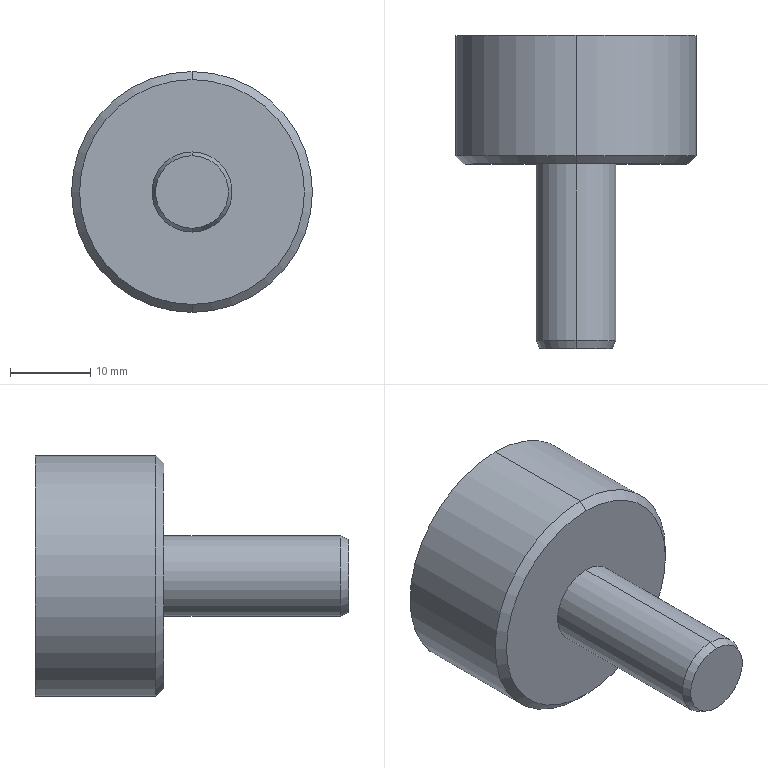Part | SolidWorks | features BaseBody 1 | 1 solid | 11 faces | box 30 x 39 x 30 mm | volume 13063 mm3 | cylinder 4 | cone 4 | plane 3 | commonest cylinder face diameters 10 x2 30 x2
STEP:
#1=CARTESIAN_POINT('',(418.,-39.,232.121));
#2=VERTEX_POINT('',#1);
#3=CARTESIAN_POINT('',(418.,-39.,262.121));
#4=VERTEX_POINT('',#3);
#5=CARTESIAN_POINT('',(418.,-39.,247.121));
#6=DIRECTION('',(0.,-1.,0.));
#7=DIRECTION('',(0.,0.,-1.));
#8=AXIS2_PLACEMENT_3D('',#5,#6,#7);
#9=CIRCLE('',#8,15.);
#10=EDGE_CURVE('',#2,#4,#9,.T.);
#11=ORIENTED_EDGE('',*,*,#10,.T.);
#12=CARTESIAN_POINT('',(418.,-54.,262.121));
#13=VERTEX_POINT('',#12);
#14=CARTESIAN_POINT('',(418.,-78.,262.121));
#15=DIRECTION('',(0.,-1.,0.));
#16=VECTOR('',#15,1000.);
#17=LINE('',#14,#16);
#18=EDGE_CURVE('',#4,#13,#17,.T.);
#19=ORIENTED_EDGE('',*,*,#18,.T.);
#20=CARTESIAN_POINT('',(418.,-54.,232.121));
#21=VERTEX_POINT('',#20);
#22=CARTESIAN_POINT('',(418.,-54.,247.121));
#23=DIRECTION('',(0.,1.,0.));
#24=DIRECTION('',(0.,0.,-1.));
#25=AXIS2_PLACEMENT_3D('',#22,#23,#24);
#26=CIRCLE('',#25,15.);
#27=EDGE_CURVE('',#13,#21,#26,.T.);
#28=ORIENTED_EDGE('',*,*,#27,.T.);
#29=CARTESIAN_POINT('',(418.,-78.,232.121));
#30=DIRECTION('',(0.,-1.,0.));
#31=VECTOR('',#30,1000.);
#32=LINE('',#29,#31);
#33=EDGE_CURVE('',#2,#21,#32,.T.);
#34=ORIENTED_EDGE('',*,*,#33,.F.);
#35=EDGE_LOOP('',(#11,#19,#28,#34));
#36=FACE_OUTER_BOUND('',#35,.T.);
#37=CARTESIAN_POINT('',(418.,-78.,247.121));
#38=DIRECTION('',(0.,-1.,0.));
#39=DIRECTION('',(0.,0.,-1.));
#40=AXIS2_PLACEMENT_3D('',#37,#38,#39);
#41=CYLINDRICAL_SURFACE('',#40,15.);
#42=ADVANCED_FACE('',(#36),#41,.T.);
#43=CARTESIAN_POINT('',(418.,-55.,261.121));
#44=VERTEX_POINT('',#43);
#45=CARTESIAN_POINT('',(418.,-55.,233.121));
#46=VERTEX_POINT('',#45);
#47=CARTESIAN_POINT('',(418.,-55.,247.121));
#48=DIRECTION('',(0.,1.,0.));
#49=DIRECTION('',(0.,0.,1.));
#50=AXIS2_PLACEMENT_3D('',#47,#48,#49);
#51=CIRCLE('',#50,14.);
#52=EDGE_CURVE('',#44,#46,#51,.T.);
#53=ORIENTED_EDGE('',*,*,#52,.T.);
#54=CARTESIAN_POINT('',(418.,-54.,232.121));
#55=DIRECTION('',(0.,0.7071,-0.7071));
#56=VECTOR('',#55,1000.);
#57=LINE('',#54,#56);
#58=EDGE_CURVE('',#46,#21,#57,.T.);
#59=ORIENTED_EDGE('',*,*,#58,.T.);
#60=ORIENTED_EDGE('',*,*,#27,.F.);
#61=CARTESIAN_POINT('',(418.,-54.,262.121));
#62=DIRECTION('',(0.,0.7071,0.7071));
#63=VECTOR('',#62,1000.);
#64=LINE('',#61,#63);
#65=EDGE_CURVE('',#44,#13,#64,.T.);
#66=ORIENTED_EDGE('',*,*,#65,.F.);
#67=EDGE_LOOP('',(#53,#59,#60,#66));
#68=FACE_OUTER_BOUND('',#67,.T.);
#69=CARTESIAN_POINT('',(418.,-54.,247.121));
#70=DIRECTION('',(0.,1.,0.));
#71=DIRECTION('',(0.,0.,1.));
#72=AXIS2_PLACEMENT_3D('',#69,#70,#71);
#73=CONICAL_SURFACE('',#72,15.,0.7854);
#74=ADVANCED_FACE('',(#68),#73,.T.);
#75=CARTESIAN_POINT('',(418.,-55.,252.121));
#76=VERTEX_POINT('',#75);
#77=CARTESIAN_POINT('',(418.,-55.,242.121));
#78=VERTEX_POINT('',#77);
#79=CARTESIAN_POINT('',(418.,-55.,247.121));
#80=DIRECTION('',(0.,1.,0.));
#81=DIRECTION('',(0.,0.,-1.));
#82=AXIS2_PLACEMENT_3D('',#79,#80,#81);
#83=CIRCLE('',#82,5.);
#84=EDGE_CURVE('',#76,#78,#83,.T.);
#85=ORIENTED_EDGE('',*,*,#84,.F.);
#86=CARTESIAN_POINT('',(418.,-77.,252.121));
#87=VERTEX_POINT('',#86);
#88=CARTESIAN_POINT('',(418.,-78.,252.121));
#89=DIRECTION('',(0.,-1.,0.));
#90=VECTOR('',#89,1000.);
#91=LINE('',#88,#90);
#92=EDGE_CURVE('',#76,#87,#91,.T.);
#93=ORIENTED_EDGE('',*,*,#92,.T.);
#94=CARTESIAN_POINT('',(418.,-77.,242.121));
#95=VERTEX_POINT('',#94);
#96=CARTESIAN_POINT('',(418.,-77.,247.121));
#97=DIRECTION('',(0.,1.,0.));
#98=DIRECTION('',(0.,0.,-1.));
#99=AXIS2_PLACEMENT_3D('',#96,#97,#98);
#100=CIRCLE('',#99,5.);
#101=EDGE_CURVE('',#87,#95,#100,.T.);
#102=ORIENTED_EDGE('',*,*,#101,.T.);
#103=CARTESIAN_POINT('',(418.,-78.,242.121));
#104=DIRECTION('',(0.,-1.,0.));
#105=VECTOR('',#104,1000.);
#106=LINE('',#103,#105);
#107=EDGE_CURVE('',#78,#95,#106,.T.);
#108=ORIENTED_EDGE('',*,*,#107,.F.);
#109=EDGE_LOOP('',(#85,#93,#102,#108));
#110=FACE_OUTER_BOUND('',#109,.T.);
#111=CARTESIAN_POINT('',(418.,-78.,247.121));
#112=DIRECTION('',(0.,-1.,0.));
#113=DIRECTION('',(0.,0.,-1.));
#114=AXIS2_PLACEMENT_3D('',#111,#112,#113);
#115=CYLINDRICAL_SURFACE('',#114,5.);
#116=ADVANCED_FACE('',(#110),#115,.T.);
#117=CARTESIAN_POINT('',(418.,-78.,251.655));
#118=VERTEX_POINT('',#117);
#119=CARTESIAN_POINT('',(418.,-78.,242.587));
#120=VERTEX_POINT('',#119);
#121=CARTESIAN_POINT('',(418.,-78.,247.121));
#122=DIRECTION('',(0.,1.,0.));
#123=DIRECTION('',(0.,0.,1.));
#124=AXIS2_PLACEMENT_3D('',#121,#122,#123);
#125=CIRCLE('',#124,4.534);
#126=EDGE_CURVE('',#118,#120,#125,.T.);
#127=ORIENTED_EDGE('',*,*,#126,.T.);
#128=CARTESIAN_POINT('',(418.,-77.,242.121));
#129=DIRECTION('',(0.,0.9063,-0.4226));
#130=VECTOR('',#129,1000.);
#131=LINE('',#128,#130);
#132=EDGE_CURVE('',#120,#95,#131,.T.);
#133=ORIENTED_EDGE('',*,*,#132,.T.);
#134=ORIENTED_EDGE('',*,*,#101,.F.);
#135=CARTESIAN_POINT('',(418.,-77.,252.121));
#136=DIRECTION('',(0.,0.9063,0.4226));
#137=VECTOR('',#136,1000.);
#138=LINE('',#135,#137);
#139=EDGE_CURVE('',#118,#87,#138,.T.);
#140=ORIENTED_EDGE('',*,*,#139,.F.);
#141=EDGE_LOOP('',(#127,#133,#134,#140));
#142=FACE_OUTER_BOUND('',#141,.T.);
#143=CARTESIAN_POINT('',(418.,-77.,247.121));
#144=DIRECTION('',(0.,1.,0.));
#145=DIRECTION('',(0.,0.,1.));
#146=AXIS2_PLACEMENT_3D('',#143,#144,#145);
#147=CONICAL_SURFACE('',#146,5.,0.4363);
#148=ADVANCED_FACE('',(#142),#147,.T.);
#149=ORIENTED_EDGE('',*,*,#18,.F.);
#150=CARTESIAN_POINT('',(418.,-39.,247.121));
#151=DIRECTION('',(0.,-1.,0.));
#152=DIRECTION('',(0.,0.,-1.));
#153=AXIS2_PLACEMENT_3D('',#150,#151,#152);
#154=CIRCLE('',#153,15.);
#155=EDGE_CURVE('',#4,#2,#154,.T.);
#156=ORIENTED_EDGE('',*,*,#155,.T.);
#157=ORIENTED_EDGE('',*,*,#33,.T.);
#158=CARTESIAN_POINT('',(418.,-54.,247.121));
#159=DIRECTION('',(0.,1.,0.));
#160=DIRECTION('',(0.,0.,-1.));
#161=AXIS2_PLACEMENT_3D('',#158,#159,#160);
#162=CIRCLE('',#161,15.);
#163=EDGE_CURVE('',#21,#13,#162,.T.);
#164=ORIENTED_EDGE('',*,*,#163,.T.);
#165=EDGE_LOOP('',(#149,#156,#157,#164));
#166=FACE_OUTER_BOUND('',#165,.T.);
#167=CARTESIAN_POINT('',(418.,-78.,247.121));
#168=DIRECTION('',(0.,-1.,0.));
#169=DIRECTION('',(0.,0.,-1.));
#170=AXIS2_PLACEMENT_3D('',#167,#168,#169);
#171=CYLINDRICAL_SURFACE('',#170,15.);
#172=ADVANCED_FACE('',(#166),#171,.T.);
#173=ORIENTED_EDGE('',*,*,#58,.F.);
#174=CARTESIAN_POINT('',(418.,-55.,247.121));
#175=DIRECTION('',(0.,1.,0.));
#176=DIRECTION('',(0.,0.,1.));
#177=AXIS2_PLACEMENT_3D('',#174,#175,#176);
#178=CIRCLE('',#177,14.);
#179=EDGE_CURVE('',#46,#44,#178,.T.);
#180=ORIENTED_EDGE('',*,*,#179,.T.);
#181=ORIENTED_EDGE('',*,*,#65,.T.);
#182=ORIENTED_EDGE('',*,*,#163,.F.);
#183=EDGE_LOOP('',(#173,#180,#181,#182));
#184=FACE_OUTER_BOUND('',#183,.T.);
#185=CARTESIAN_POINT('',(418.,-54.,247.121));
#186=DIRECTION('',(0.,1.,0.));
#187=DIRECTION('',(0.,0.,1.));
#188=AXIS2_PLACEMENT_3D('',#185,#186,#187);
#189=CONICAL_SURFACE('',#188,15.,0.7854);
#190=ADVANCED_FACE('',(#184),#189,.T.);
#191=ORIENTED_EDGE('',*,*,#10,.F.);
#192=ORIENTED_EDGE('',*,*,#155,.F.);
#193=EDGE_LOOP('',(#191,#192));
#194=FACE_OUTER_BOUND('',#193,.T.);
#195=CARTESIAN_POINT('',(418.,-39.,247.121));
#196=DIRECTION('',(0.,1.,0.));
#197=DIRECTION('',(0.,0.,1.));
#198=AXIS2_PLACEMENT_3D('',#195,#196,#197);
#199=PLANE('',#198);
#200=ADVANCED_FACE('',(#194),#199,.T.);
#201=CARTESIAN_POINT('',(418.,-55.,247.121));
#202=DIRECTION('',(0.,1.,0.));
#203=DIRECTION('',(0.,0.,-1.));
#204=AXIS2_PLACEMENT_3D('',#201,#202,#203);
#205=CIRCLE('',#204,5.);
#206=EDGE_CURVE('',#78,#76,#205,.T.);
#207=ORIENTED_EDGE('',*,*,#206,.T.);
#208=ORIENTED_EDGE('',*,*,#84,.T.);
#209=EDGE_LOOP('',(#207,#208));
#210=FACE_BOUND('',#209,.T.);
#211=ORIENTED_EDGE('',*,*,#52,.F.);
#212=ORIENTED_EDGE('',*,*,#179,.F.);
#213=EDGE_LOOP('',(#211,#212));
#214=FACE_OUTER_BOUND('',#213,.T.);
#215=CARTESIAN_POINT('',(403.,-55.,247.121));
#216=DIRECTION('',(0.,-1.,0.));
#217=DIRECTION('',(0.,0.,-1.));
#218=AXIS2_PLACEMENT_3D('',#215,#216,#217);
#219=PLANE('',#218);
#220=ADVANCED_FACE('',(#210,#214),#219,.T.);
#221=ORIENTED_EDGE('',*,*,#92,.F.);
#222=ORIENTED_EDGE('',*,*,#206,.F.);
#223=ORIENTED_EDGE('',*,*,#107,.T.);
#224=CARTESIAN_POINT('',(418.,-77.,247.121));
#225=DIRECTION('',(0.,1.,0.));
#226=DIRECTION('',(0.,0.,-1.));
#227=AXIS2_PLACEMENT_3D('',#224,#225,#226);
#228=CIRCLE('',#227,5.);
#229=EDGE_CURVE('',#95,#87,#228,.T.);
#230=ORIENTED_EDGE('',*,*,#229,.T.);
#231=EDGE_LOOP('',(#221,#222,#223,#230));
#232=FACE_OUTER_BOUND('',#231,.T.);
#233=CARTESIAN_POINT('',(418.,-78.,247.121));
#234=DIRECTION('',(0.,-1.,0.));
#235=DIRECTION('',(0.,0.,-1.));
#236=AXIS2_PLACEMENT_3D('',#233,#234,#235);
#237=CYLINDRICAL_SURFACE('',#236,5.);
#238=ADVANCED_FACE('',(#232),#237,.T.);
#239=ORIENTED_EDGE('',*,*,#132,.F.);
#240=CARTESIAN_POINT('',(418.,-78.,247.121));
#241=DIRECTION('',(0.,1.,0.));
#242=DIRECTION('',(0.,0.,1.));
#243=AXIS2_PLACEMENT_3D('',#240,#241,#242);
#244=CIRCLE('',#243,4.534);
#245=EDGE_CURVE('',#120,#118,#244,.T.);
#246=ORIENTED_EDGE('',*,*,#245,.T.);
#247=ORIENTED_EDGE('',*,*,#139,.T.);
#248=ORIENTED_EDGE('',*,*,#229,.F.);
#249=EDGE_LOOP('',(#239,#246,#247,#248));
#250=FACE_OUTER_BOUND('',#249,.T.);
#251=CARTESIAN_POINT('',(418.,-77.,247.121));
#252=DIRECTION('',(0.,1.,0.));
#253=DIRECTION('',(0.,0.,1.));
#254=AXIS2_PLACEMENT_3D('',#251,#252,#253);
#255=CONICAL_SURFACE('',#254,5.,0.4363);
#256=ADVANCED_FACE('',(#250),#255,.T.);
#257=ORIENTED_EDGE('',*,*,#126,.F.);
#258=ORIENTED_EDGE('',*,*,#245,.F.);
#259=EDGE_LOOP('',(#257,#258));
#260=FACE_OUTER_BOUND('',#259,.T.);
#261=CARTESIAN_POINT('',(413.,-78.,247.121));
#262=DIRECTION('',(0.,-1.,0.));
#263=DIRECTION('',(0.,0.,-1.));
#264=AXIS2_PLACEMENT_3D('',#261,#262,#263);
#265=PLANE('',#264);
#266=ADVANCED_FACE('',(#260),#265,.T.);
#267=CLOSED_SHELL('',(#42,#74,#116,#148,#172,#190,#200,#220,#238,#256,#266));
#268=MANIFOLD_SOLID_BREP('',#267);
#269=CARTESIAN_POINT('',(0.,0.,0.));
#270=DIRECTION('',(0.,0.,1.));
#271=DIRECTION('',(1.,0.,0.));
#272=AXIS2_PLACEMENT_3D('',#269,#270,#271);
#273=(LENGTH_UNIT()NAMED_UNIT(*)SI_UNIT(.MILLI.,.METRE.));
#274=UNCERTAINTY_MEASURE_WITH_UNIT(LENGTH_MEASURE(0.00001),#273,'','');
#275=(NAMED_UNIT(*)PLANE_ANGLE_UNIT()SI_UNIT($,.RADIAN.));
#276=(NAMED_UNIT(*)SI_UNIT($,.STERADIAN.)SOLID_ANGLE_UNIT());
#277=(GEOMETRIC_REPRESENTATION_CONTEXT(3)GLOBAL_UNCERTAINTY_ASSIGNED_CONTEXT((#274))GLOBAL_UNIT_ASSIGNED_CONTEXT((#273,#275,#276))REPRESENTATION_CONTEXT('',''));
#278=ADVANCED_BREP_SHAPE_REPRESENTATION('',(#268,#272),#277);